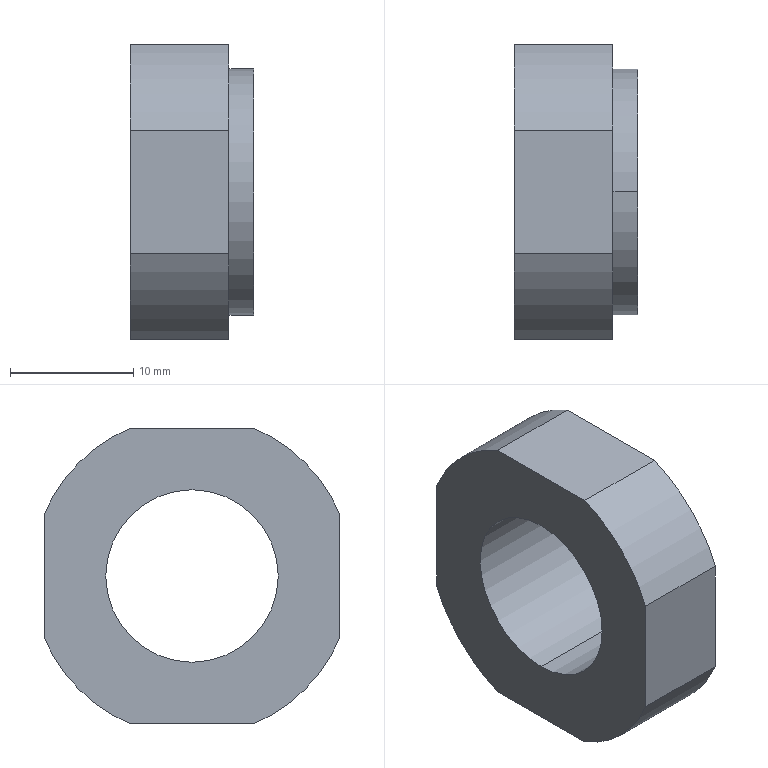Part | STEP file | PN_0054 locking nut | 1 solid | 15 faces | box 10 x 24 x 24 mm | volume 3121 mm3 | cylinder 8 | plane 7 | commonest cylinder face diameters 26 x4 14 x2 20 x2
STEP:
#1=CARTESIAN_POINT('',(0.,0.,0.));
#2=DIRECTION('',(0.,0.,1.));
#3=DIRECTION('',(1.,0.,0.));
#4=AXIS2_PLACEMENT_3D('',#1,#2,#3);
#5=CARTESIAN_POINT('',(-10.,0.,-7.));
#6=VERTEX_POINT('',#5);
#7=CARTESIAN_POINT('',(0.,0.,-7.));
#8=VERTEX_POINT('',#7);
#9=CARTESIAN_POINT('',(-10.,0.,-7.));
#10=DIRECTION('',(1.,0.,0.));
#11=VECTOR('',#10,1.);
#12=LINE('',#9,#11);
#13=CARTESIAN_POINT('',(-10.,0.,0.));
#14=DIRECTION('',(1.,0.,0.));
#15=DIRECTION('',(0.,0.,-1.));
#16=AXIS2_PLACEMENT_3D('',#13,#14,#15);
#17=CYLINDRICAL_SURFACE('',#16,7.);
#18=CARTESIAN_POINT('',(6.283,0.));
#19=DIRECTION('',(0.,1.));
#20=VECTOR('',#19,1.);
#21=LINE('',#18,#20);
#22=(GEOMETRIC_REPRESENTATION_CONTEXT(2)PARAMETRIC_REPRESENTATION_CONTEXT()REPRESENTATION_CONTEXT('',''));
#23=DEFINITIONAL_REPRESENTATION('',(#21),#22);
#24=PCURVE('',#17,#23);
#25=CARTESIAN_POINT('',(-10.,0.,0.));
#26=DIRECTION('',(1.,0.,0.));
#27=DIRECTION('',(0.,0.,-1.));
#28=AXIS2_PLACEMENT_3D('',#25,#26,#27);
#29=CYLINDRICAL_SURFACE('',#28,7.);
#30=CARTESIAN_POINT('',(0.,0.));
#31=DIRECTION('',(0.,1.));
#32=VECTOR('',#31,1.);
#33=LINE('',#30,#32);
#34=(GEOMETRIC_REPRESENTATION_CONTEXT(2)PARAMETRIC_REPRESENTATION_CONTEXT()REPRESENTATION_CONTEXT('',''));
#35=DEFINITIONAL_REPRESENTATION('',(#33),#34);
#36=PCURVE('',#29,#35);
#37=SURFACE_CURVE('',#12,(#24,#36),.PCURVE_S1.);
#38=EDGE_CURVE('',#6,#8,#37,.T.);
#39=ORIENTED_EDGE('',*,*,#38,.T.);
#40=CARTESIAN_POINT('',(0.,0.,7.));
#41=VERTEX_POINT('',#40);
#42=CARTESIAN_POINT('',(0.,0.,0.));
#43=DIRECTION('',(1.,0.,0.));
#44=DIRECTION('',(0.,0.,-1.));
#45=AXIS2_PLACEMENT_3D('',#42,#43,#44);
#46=CIRCLE('',#45,7.);
#47=CARTESIAN_POINT('',(0.,10.));
#48=DIRECTION('',(1.,0.));
#49=VECTOR('',#48,1.);
#50=LINE('',#47,#49);
#51=(GEOMETRIC_REPRESENTATION_CONTEXT(2)PARAMETRIC_REPRESENTATION_CONTEXT()REPRESENTATION_CONTEXT('',''));
#52=DEFINITIONAL_REPRESENTATION('',(#50),#51);
#53=PCURVE('',#17,#52);
#54=CARTESIAN_POINT('',(0.,0.,0.));
#55=DIRECTION('',(1.,0.,0.));
#56=DIRECTION('',(0.,0.,-1.));
#57=AXIS2_PLACEMENT_3D('',#54,#55,#56);
#58=PLANE('',#57);
#59=CARTESIAN_POINT('',(0.,0.));
#60=DIRECTION('',(1.,0.));
#61=AXIS2_PLACEMENT_2D('',#59,#60);
#62=CIRCLE('',#61,7.);
#63=(GEOMETRIC_REPRESENTATION_CONTEXT(2)PARAMETRIC_REPRESENTATION_CONTEXT()REPRESENTATION_CONTEXT('',''));
#64=DEFINITIONAL_REPRESENTATION('',(#62),#63);
#65=PCURVE('',#58,#64);
#66=SURFACE_CURVE('',#46,(#53,#65),.PCURVE_S1.);
#67=EDGE_CURVE('',#41,#8,#66,.T.);
#68=ORIENTED_EDGE('',*,*,#67,.F.);
#69=CARTESIAN_POINT('',(-10.,0.,7.));
#70=VERTEX_POINT('',#69);
#71=CARTESIAN_POINT('',(-10.,0.,7.));
#72=DIRECTION('',(1.,0.,0.));
#73=VECTOR('',#72,1.);
#74=LINE('',#71,#73);
#75=CARTESIAN_POINT('',(3.142,0.));
#76=DIRECTION('',(0.,1.));
#77=VECTOR('',#76,1.);
#78=LINE('',#75,#77);
#79=(GEOMETRIC_REPRESENTATION_CONTEXT(2)PARAMETRIC_REPRESENTATION_CONTEXT()REPRESENTATION_CONTEXT('',''));
#80=DEFINITIONAL_REPRESENTATION('',(#78),#79);
#81=PCURVE('',#17,#80);
#82=CARTESIAN_POINT('',(3.142,0.));
#83=DIRECTION('',(0.,1.));
#84=VECTOR('',#83,1.);
#85=LINE('',#82,#84);
#86=(GEOMETRIC_REPRESENTATION_CONTEXT(2)PARAMETRIC_REPRESENTATION_CONTEXT()REPRESENTATION_CONTEXT('',''));
#87=DEFINITIONAL_REPRESENTATION('',(#85),#86);
#88=PCURVE('',#29,#87);
#89=SURFACE_CURVE('',#74,(#81,#88),.PCURVE_S1.);
#90=EDGE_CURVE('',#70,#41,#89,.T.);
#91=ORIENTED_EDGE('',*,*,#90,.F.);
#92=CARTESIAN_POINT('',(-10.,0.,0.));
#93=DIRECTION('',(1.,0.,0.));
#94=DIRECTION('',(0.,0.,-1.));
#95=AXIS2_PLACEMENT_3D('',#92,#93,#94);
#96=CIRCLE('',#95,7.);
#97=CARTESIAN_POINT('',(0.,0.));
#98=DIRECTION('',(1.,0.));
#99=VECTOR('',#98,1.);
#100=LINE('',#97,#99);
#101=(GEOMETRIC_REPRESENTATION_CONTEXT(2)PARAMETRIC_REPRESENTATION_CONTEXT()REPRESENTATION_CONTEXT('',''));
#102=DEFINITIONAL_REPRESENTATION('',(#100),#101);
#103=PCURVE('',#17,#102);
#104=CARTESIAN_POINT('',(-10.,13.,0.));
#105=DIRECTION('',(-1.,0.,0.));
#106=DIRECTION('',(0.,0.,1.));
#107=AXIS2_PLACEMENT_3D('',#104,#105,#106);
#108=PLANE('',#107);
#109=CARTESIAN_POINT('',(-7.,-13.));
#110=CARTESIAN_POINT('',(-7.,-0.8756));
#111=CARTESIAN_POINT('',(3.5,-6.938));
#112=CARTESIAN_POINT('',(14.,-13.));
#113=CARTESIAN_POINT('',(3.5,-19.062));
#114=CARTESIAN_POINT('',(-7.,-25.124));
#115=CARTESIAN_POINT('',(-7.,-13.));
#116=(BOUNDED_CURVE()B_SPLINE_CURVE(2,(#109,#110,#111,#112,#113,#114,#115),.UNSPECIFIED.,.T.,.F.)B_SPLINE_CURVE_WITH_KNOTS((1,2,2,2,2,1),(-2.094,0.,2.094,4.189,6.283,8.378),.UNSPECIFIED.)CURVE()GEOMETRIC_REPRESENTATION_ITEM()RATIONAL_B_SPLINE_CURVE((1.,0.5,1.,0.5,1.,0.5,1.))REPRESENTATION_ITEM(''));
#117=(GEOMETRIC_REPRESENTATION_CONTEXT(2)PARAMETRIC_REPRESENTATION_CONTEXT()REPRESENTATION_CONTEXT('',''));
#118=DEFINITIONAL_REPRESENTATION('',(#116),#117);
#119=PCURVE('',#108,#118);
#120=SURFACE_CURVE('',#96,(#103,#119),.PCURVE_S1.);
#121=EDGE_CURVE('',#70,#6,#120,.T.);
#122=ORIENTED_EDGE('',*,*,#121,.T.);
#123=EDGE_LOOP('',(#39,#68,#91,#122));
#124=FACE_BOUND('',#123,.F.);
#125=ADVANCED_FACE('',(#124),#17,.F.);
#126=CARTESIAN_POINT('',(-2.,0.,-10.));
#127=VERTEX_POINT('',#126);
#128=CARTESIAN_POINT('',(-2.,0.,10.));
#129=VERTEX_POINT('',#128);
#130=CARTESIAN_POINT('',(-2.,0.,0.));
#131=DIRECTION('',(1.,0.,0.));
#132=DIRECTION('',(0.,0.,-1.));
#133=AXIS2_PLACEMENT_3D('',#130,#131,#132);
#134=CIRCLE('',#133,10.);
#135=CARTESIAN_POINT('',(0.,0.,0.));
#136=DIRECTION('',(1.,0.,0.));
#137=DIRECTION('',(0.,0.,-1.));
#138=AXIS2_PLACEMENT_3D('',#135,#136,#137);
#139=CYLINDRICAL_SURFACE('',#138,10.);
#140=CARTESIAN_POINT('',(0.,-2.));
#141=DIRECTION('',(1.,0.));
#142=VECTOR('',#141,1.);
#143=LINE('',#140,#142);
#144=(GEOMETRIC_REPRESENTATION_CONTEXT(2)PARAMETRIC_REPRESENTATION_CONTEXT()REPRESENTATION_CONTEXT('',''));
#145=DEFINITIONAL_REPRESENTATION('',(#143),#144);
#146=PCURVE('',#139,#145);
#147=CARTESIAN_POINT('',(-2.,10.,0.));
#148=DIRECTION('',(1.,0.,0.));
#149=DIRECTION('',(0.,0.,-1.));
#150=AXIS2_PLACEMENT_3D('',#147,#148,#149);
#151=PLANE('',#150);
#152=CARTESIAN_POINT('',(0.,-10.));
#153=DIRECTION('',(1.,0.));
#154=AXIS2_PLACEMENT_2D('',#152,#153);
#155=CIRCLE('',#154,10.);
#156=(GEOMETRIC_REPRESENTATION_CONTEXT(2)PARAMETRIC_REPRESENTATION_CONTEXT()REPRESENTATION_CONTEXT('',''));
#157=DEFINITIONAL_REPRESENTATION('',(#155),#156);
#158=PCURVE('',#151,#157);
#159=SURFACE_CURVE('',#134,(#146,#158),.PCURVE_S1.);
#160=EDGE_CURVE('',#127,#129,#159,.T.);
#161=ORIENTED_EDGE('',*,*,#160,.T.);
#162=CARTESIAN_POINT('',(0.,0.,10.));
#163=VERTEX_POINT('',#162);
#164=CARTESIAN_POINT('',(0.,0.,10.));
#165=DIRECTION('',(1.,0.,0.));
#166=VECTOR('',#165,1.);
#167=LINE('',#164,#166);
#168=CARTESIAN_POINT('',(3.142,0.));
#169=DIRECTION('',(0.,1.));
#170=VECTOR('',#169,1.);
#171=LINE('',#168,#170);
#172=(GEOMETRIC_REPRESENTATION_CONTEXT(2)PARAMETRIC_REPRESENTATION_CONTEXT()REPRESENTATION_CONTEXT('',''));
#173=DEFINITIONAL_REPRESENTATION('',(#171),#172);
#174=PCURVE('',#139,#173);
#175=CARTESIAN_POINT('',(0.,0.,0.));
#176=DIRECTION('',(1.,0.,0.));
#177=DIRECTION('',(0.,0.,-1.));
#178=AXIS2_PLACEMENT_3D('',#175,#176,#177);
#179=CYLINDRICAL_SURFACE('',#178,10.);
#180=CARTESIAN_POINT('',(3.142,0.));
#181=DIRECTION('',(0.,1.));
#182=VECTOR('',#181,1.);
#183=LINE('',#180,#182);
#184=(GEOMETRIC_REPRESENTATION_CONTEXT(2)PARAMETRIC_REPRESENTATION_CONTEXT()REPRESENTATION_CONTEXT('',''));
#185=DEFINITIONAL_REPRESENTATION('',(#183),#184);
#186=PCURVE('',#179,#185);
#187=SURFACE_CURVE('',#167,(#174,#186),.PCURVE_S1.);
#188=EDGE_CURVE('',#129,#163,#187,.T.);
#189=ORIENTED_EDGE('',*,*,#188,.T.);
#190=CARTESIAN_POINT('',(0.,0.,-10.));
#191=VERTEX_POINT('',#190);
#192=CARTESIAN_POINT('',(0.,0.,0.));
#193=DIRECTION('',(1.,0.,0.));
#194=DIRECTION('',(0.,0.,-1.));
#195=AXIS2_PLACEMENT_3D('',#192,#193,#194);
#196=CIRCLE('',#195,10.);
#197=CARTESIAN_POINT('',(0.,0.));
#198=DIRECTION('',(1.,0.));
#199=VECTOR('',#198,1.);
#200=LINE('',#197,#199);
#201=(GEOMETRIC_REPRESENTATION_CONTEXT(2)PARAMETRIC_REPRESENTATION_CONTEXT()REPRESENTATION_CONTEXT('',''));
#202=DEFINITIONAL_REPRESENTATION('',(#200),#201);
#203=PCURVE('',#139,#202);
#204=CARTESIAN_POINT('',(0.,0.));
#205=DIRECTION('',(1.,0.));
#206=AXIS2_PLACEMENT_2D('',#204,#205);
#207=CIRCLE('',#206,10.);
#208=(GEOMETRIC_REPRESENTATION_CONTEXT(2)PARAMETRIC_REPRESENTATION_CONTEXT()REPRESENTATION_CONTEXT('',''));
#209=DEFINITIONAL_REPRESENTATION('',(#207),#208);
#210=PCURVE('',#58,#209);
#211=SURFACE_CURVE('',#196,(#203,#210),.PCURVE_S1.);
#212=EDGE_CURVE('',#191,#163,#211,.T.);
#213=ORIENTED_EDGE('',*,*,#212,.F.);
#214=CARTESIAN_POINT('',(0.,0.,-10.));
#215=DIRECTION('',(1.,0.,0.));
#216=VECTOR('',#215,1.);
#217=LINE('',#214,#216);
#218=CARTESIAN_POINT('',(0.,0.));
#219=DIRECTION('',(0.,1.));
#220=VECTOR('',#219,1.);
#221=LINE('',#218,#220);
#222=(GEOMETRIC_REPRESENTATION_CONTEXT(2)PARAMETRIC_REPRESENTATION_CONTEXT()REPRESENTATION_CONTEXT('',''));
#223=DEFINITIONAL_REPRESENTATION('',(#221),#222);
#224=PCURVE('',#139,#223);
#225=CARTESIAN_POINT('',(6.283,0.));
#226=DIRECTION('',(0.,1.));
#227=VECTOR('',#226,1.);
#228=LINE('',#225,#227);
#229=(GEOMETRIC_REPRESENTATION_CONTEXT(2)PARAMETRIC_REPRESENTATION_CONTEXT()REPRESENTATION_CONTEXT('',''));
#230=DEFINITIONAL_REPRESENTATION('',(#228),#229);
#231=PCURVE('',#179,#230);
#232=SURFACE_CURVE('',#217,(#224,#231),.PCURVE_S1.);
#233=EDGE_CURVE('',#127,#191,#232,.T.);
#234=ORIENTED_EDGE('',*,*,#233,.F.);
#235=EDGE_LOOP('',(#161,#189,#213,#234));
#236=FACE_BOUND('',#235,.T.);
#237=ADVANCED_FACE('',(#236),#139,.T.);
#238=CARTESIAN_POINT('',(-2.,5.,12.));
#239=VERTEX_POINT('',#238);
#240=CARTESIAN_POINT('',(-10.,5.,12.));
#241=VERTEX_POINT('',#240);
#242=CARTESIAN_POINT('',(0.,5.,12.));
#243=DIRECTION('',(-1.,0.,0.));
#244=VECTOR('',#243,1.);
#245=LINE('',#242,#244);
#246=CARTESIAN_POINT('',(0.,0.,0.));
#247=DIRECTION('',(1.,0.,0.));
#248=DIRECTION('',(0.,0.,-1.));
#249=AXIS2_PLACEMENT_3D('',#246,#247,#248);
#250=CYLINDRICAL_SURFACE('',#249,13.);
#251=CARTESIAN_POINT('',(2.747,0.));
#252=DIRECTION('',(0.,-1.));
#253=VECTOR('',#252,1.);
#254=LINE('',#251,#253);
#255=(GEOMETRIC_REPRESENTATION_CONTEXT(2)PARAMETRIC_REPRESENTATION_CONTEXT()REPRESENTATION_CONTEXT('',''));
#256=DEFINITIONAL_REPRESENTATION('',(#254),#255);
#257=PCURVE('',#250,#256);
#258=CARTESIAN_POINT('',(0.,17.205,12.));
#259=DIRECTION('',(0.,0.,-1.));
#260=DIRECTION('',(0.,1.,0.));
#261=AXIS2_PLACEMENT_3D('',#258,#259,#260);
#262=PLANE('',#261);
#263=CARTESIAN_POINT('',(-12.205,0.));
#264=DIRECTION('',(0.,-1.));
#265=VECTOR('',#264,1.);
#266=LINE('',#263,#265);
#267=(GEOMETRIC_REPRESENTATION_CONTEXT(2)PARAMETRIC_REPRESENTATION_CONTEXT()REPRESENTATION_CONTEXT('',''));
#268=DEFINITIONAL_REPRESENTATION('',(#266),#267);
#269=PCURVE('',#262,#268);
#270=SURFACE_CURVE('',#245,(#257,#269),.PCURVE_S1.);
#271=EDGE_CURVE('',#239,#241,#270,.T.);
#272=ORIENTED_EDGE('',*,*,#271,.F.);
#273=CARTESIAN_POINT('',(-2.,12.,5.));
#274=VERTEX_POINT('',#273);
#275=CARTESIAN_POINT('',(-2.,0.,0.));
#276=DIRECTION('',(1.,0.,0.));
#277=DIRECTION('',(0.,0.,-1.));
#278=AXIS2_PLACEMENT_3D('',#275,#276,#277);
#279=CIRCLE('',#278,13.);
#280=CARTESIAN_POINT('',(0.,-2.));
#281=DIRECTION('',(1.,0.));
#282=VECTOR('',#281,1.);
#283=LINE('',#280,#282);
#284=(GEOMETRIC_REPRESENTATION_CONTEXT(2)PARAMETRIC_REPRESENTATION_CONTEXT()REPRESENTATION_CONTEXT('',''));
#285=DEFINITIONAL_REPRESENTATION('',(#283),#284);
#286=PCURVE('',#250,#285);
#287=CARTESIAN_POINT('',(0.,-10.));
#288=DIRECTION('',(1.,0.));
#289=AXIS2_PLACEMENT_2D('',#287,#288);
#290=CIRCLE('',#289,13.);
#291=(GEOMETRIC_REPRESENTATION_CONTEXT(2)PARAMETRIC_REPRESENTATION_CONTEXT()REPRESENTATION_CONTEXT('',''));
#292=DEFINITIONAL_REPRESENTATION('',(#290),#291);
#293=PCURVE('',#151,#292);
#294=SURFACE_CURVE('',#279,(#286,#293),.PCURVE_S1.);
#295=EDGE_CURVE('',#274,#239,#294,.T.);
#296=ORIENTED_EDGE('',*,*,#295,.F.);
#297=CARTESIAN_POINT('',(-10.,12.,5.));
#298=VERTEX_POINT('',#297);
#299=CARTESIAN_POINT('',(0.,12.,5.));
#300=DIRECTION('',(1.,0.,0.));
#301=VECTOR('',#300,1.);
#302=LINE('',#299,#301);
#303=CARTESIAN_POINT('',(1.966,0.));
#304=DIRECTION('',(0.,1.));
#305=VECTOR('',#304,1.);
#306=LINE('',#303,#305);
#307=(GEOMETRIC_REPRESENTATION_CONTEXT(2)PARAMETRIC_REPRESENTATION_CONTEXT()REPRESENTATION_CONTEXT('',''));
#308=DEFINITIONAL_REPRESENTATION('',(#306),#307);
#309=PCURVE('',#250,#308);
#310=CARTESIAN_POINT('',(0.,12.,-20.296));
#311=DIRECTION('',(0.,-1.,0.));
#312=DIRECTION('',(0.,0.,-1.));
#313=AXIS2_PLACEMENT_3D('',#310,#311,#312);
#314=PLANE('',#313);
#315=CARTESIAN_POINT('',(-25.296,0.));
#316=DIRECTION('',(0.,1.));
#317=VECTOR('',#316,1.);
#318=LINE('',#315,#317);
#319=(GEOMETRIC_REPRESENTATION_CONTEXT(2)PARAMETRIC_REPRESENTATION_CONTEXT()REPRESENTATION_CONTEXT('',''));
#320=DEFINITIONAL_REPRESENTATION('',(#318),#319);
#321=PCURVE('',#314,#320);
#322=SURFACE_CURVE('',#302,(#309,#321),.PCURVE_S1.);
#323=EDGE_CURVE('',#298,#274,#322,.T.);
#324=ORIENTED_EDGE('',*,*,#323,.F.);
#325=CARTESIAN_POINT('',(-10.,0.,0.));
#326=DIRECTION('',(1.,0.,0.));
#327=DIRECTION('',(0.,0.,-1.));
#328=AXIS2_PLACEMENT_3D('',#325,#326,#327);
#329=CIRCLE('',#328,13.);
#330=CARTESIAN_POINT('',(0.,-10.));
#331=DIRECTION('',(1.,0.));
#332=VECTOR('',#331,1.);
#333=LINE('',#330,#332);
#334=(GEOMETRIC_REPRESENTATION_CONTEXT(2)PARAMETRIC_REPRESENTATION_CONTEXT()REPRESENTATION_CONTEXT('',''));
#335=DEFINITIONAL_REPRESENTATION('',(#333),#334);
#336=PCURVE('',#250,#335);
#337=CARTESIAN_POINT('',(-13.,-13.));
#338=CARTESIAN_POINT('',(-13.,9.517));
#339=CARTESIAN_POINT('',(6.5,-1.742));
#340=CARTESIAN_POINT('',(26.,-13.));
#341=CARTESIAN_POINT('',(6.5,-24.258));
#342=CARTESIAN_POINT('',(-13.,-35.517));
#343=CARTESIAN_POINT('',(-13.,-13.));
#344=(BOUNDED_CURVE()B_SPLINE_CURVE(2,(#337,#338,#339,#340,#341,#342,#343),.UNSPECIFIED.,.T.,.F.)B_SPLINE_CURVE_WITH_KNOTS((1,2,2,2,2,1),(-2.094,0.,2.094,4.189,6.283,8.378),.UNSPECIFIED.)CURVE()GEOMETRIC_REPRESENTATION_ITEM()RATIONAL_B_SPLINE_CURVE((1.,0.5,1.,0.5,1.,0.5,1.))REPRESENTATION_ITEM(''));
#345=(GEOMETRIC_REPRESENTATION_CONTEXT(2)PARAMETRIC_REPRESENTATION_CONTEXT()REPRESENTATION_CONTEXT('',''));
#346=DEFINITIONAL_REPRESENTATION('',(#344),#345);
#347=PCURVE('',#108,#346);
#348=SURFACE_CURVE('',#329,(#336,#347),.PCURVE_S1.);
#349=EDGE_CURVE('',#298,#241,#348,.T.);
#350=ORIENTED_EDGE('',*,*,#349,.T.);
#351=EDGE_LOOP('',(#272,#296,#324,#350));
#352=FACE_BOUND('',#351,.T.);
#353=ADVANCED_FACE('',(#352),#250,.T.);
#354=CARTESIAN_POINT('',(-2.,-5.,-12.));
#355=VERTEX_POINT('',#354);
#356=CARTESIAN_POINT('',(-10.,-5.,-12.));
#357=VERTEX_POINT('',#356);
#358=CARTESIAN_POINT('',(0.,-5.,-12.));
#359=DIRECTION('',(-1.,0.,0.));
#360=VECTOR('',#359,1.);
#361=LINE('',#358,#360);
#362=CARTESIAN_POINT('',(0.,0.,0.));
#363=DIRECTION('',(1.,0.,0.));
#364=DIRECTION('',(0.,0.,-1.));
#365=AXIS2_PLACEMENT_3D('',#362,#363,#364);
#366=CYLINDRICAL_SURFACE('',#365,13.);
#367=CARTESIAN_POINT('',(5.888,0.));
#368=DIRECTION('',(0.,-1.));
#369=VECTOR('',#368,1.);
#370=LINE('',#367,#369);
#371=(GEOMETRIC_REPRESENTATION_CONTEXT(2)PARAMETRIC_REPRESENTATION_CONTEXT()REPRESENTATION_CONTEXT('',''));
#372=DEFINITIONAL_REPRESENTATION('',(#370),#371);
#373=PCURVE('',#366,#372);
#374=CARTESIAN_POINT('',(0.,17.205,-12.));
#375=DIRECTION('',(0.,0.,1.));
#376=DIRECTION('',(0.,-1.,0.));
#377=AXIS2_PLACEMENT_3D('',#374,#375,#376);
#378=PLANE('',#377);
#379=CARTESIAN_POINT('',(22.205,0.));
#380=DIRECTION('',(0.,-1.));
#381=VECTOR('',#380,1.);
#382=LINE('',#379,#381);
#383=(GEOMETRIC_REPRESENTATION_CONTEXT(2)PARAMETRIC_REPRESENTATION_CONTEXT()REPRESENTATION_CONTEXT('',''));
#384=DEFINITIONAL_REPRESENTATION('',(#382),#383);
#385=PCURVE('',#378,#384);
#386=SURFACE_CURVE('',#361,(#373,#385),.PCURVE_S1.);
#387=EDGE_CURVE('',#355,#357,#386,.T.);
#388=ORIENTED_EDGE('',*,*,#387,.F.);
#389=CARTESIAN_POINT('',(-2.,-12.,-5.));
#390=VERTEX_POINT('',#389);
#391=CARTESIAN_POINT('',(-2.,0.,0.));
#392=DIRECTION('',(1.,0.,0.));
#393=DIRECTION('',(0.,0.,-1.));
#394=AXIS2_PLACEMENT_3D('',#391,#392,#393);
#395=CIRCLE('',#394,13.);
#396=CARTESIAN_POINT('',(0.,-2.));
#397=DIRECTION('',(1.,0.));
#398=VECTOR('',#397,1.);
#399=LINE('',#396,#398);
#400=(GEOMETRIC_REPRESENTATION_CONTEXT(2)PARAMETRIC_REPRESENTATION_CONTEXT()REPRESENTATION_CONTEXT('',''));
#401=DEFINITIONAL_REPRESENTATION('',(#399),#400);
#402=PCURVE('',#366,#401);
#403=CARTESIAN_POINT('',(0.,-10.));
#404=DIRECTION('',(1.,0.));
#405=AXIS2_PLACEMENT_2D('',#403,#404);
#406=CIRCLE('',#405,13.);
#407=(GEOMETRIC_REPRESENTATION_CONTEXT(2)PARAMETRIC_REPRESENTATION_CONTEXT()REPRESENTATION_CONTEXT('',''));
#408=DEFINITIONAL_REPRESENTATION('',(#406),#407);
#409=PCURVE('',#151,#408);
#410=SURFACE_CURVE('',#395,(#402,#409),.PCURVE_S1.);
#411=EDGE_CURVE('',#390,#355,#410,.T.);
#412=ORIENTED_EDGE('',*,*,#411,.F.);
#413=CARTESIAN_POINT('',(-10.,-12.,-5.));
#414=VERTEX_POINT('',#413);
#415=CARTESIAN_POINT('',(0.,-12.,-5.));
#416=DIRECTION('',(1.,0.,0.));
#417=VECTOR('',#416,1.);
#418=LINE('',#415,#417);
#419=CARTESIAN_POINT('',(5.107,0.));
#420=DIRECTION('',(0.,1.));
#421=VECTOR('',#420,1.);
#422=LINE('',#419,#421);
#423=(GEOMETRIC_REPRESENTATION_CONTEXT(2)PARAMETRIC_REPRESENTATION_CONTEXT()REPRESENTATION_CONTEXT('',''));
#424=DEFINITIONAL_REPRESENTATION('',(#422),#423);
#425=PCURVE('',#366,#424);
#426=CARTESIAN_POINT('',(0.,-12.,-20.296));
#427=DIRECTION('',(0.,1.,0.));
#428=DIRECTION('',(0.,0.,1.));
#429=AXIS2_PLACEMENT_3D('',#426,#427,#428);
#430=PLANE('',#429);
#431=CARTESIAN_POINT('',(15.296,0.));
#432=DIRECTION('',(0.,1.));
#433=VECTOR('',#432,1.);
#434=LINE('',#431,#433);
#435=(GEOMETRIC_REPRESENTATION_CONTEXT(2)PARAMETRIC_REPRESENTATION_CONTEXT()REPRESENTATION_CONTEXT('',''));
#436=DEFINITIONAL_REPRESENTATION('',(#434),#435);
#437=PCURVE('',#430,#436);
#438=SURFACE_CURVE('',#418,(#425,#437),.PCURVE_S1.);
#439=EDGE_CURVE('',#414,#390,#438,.T.);
#440=ORIENTED_EDGE('',*,*,#439,.F.);
#441=CARTESIAN_POINT('',(-10.,0.,0.));
#442=DIRECTION('',(1.,0.,0.));
#443=DIRECTION('',(0.,0.,-1.));
#444=AXIS2_PLACEMENT_3D('',#441,#442,#443);
#445=CIRCLE('',#444,13.);
#446=CARTESIAN_POINT('',(0.,-10.));
#447=DIRECTION('',(1.,0.));
#448=VECTOR('',#447,1.);
#449=LINE('',#446,#448);
#450=(GEOMETRIC_REPRESENTATION_CONTEXT(2)PARAMETRIC_REPRESENTATION_CONTEXT()REPRESENTATION_CONTEXT('',''));
#451=DEFINITIONAL_REPRESENTATION('',(#449),#450);
#452=PCURVE('',#366,#451);
#453=CARTESIAN_POINT('',(-13.,-13.));
#454=CARTESIAN_POINT('',(-13.,9.517));
#455=CARTESIAN_POINT('',(6.5,-1.742));
#456=CARTESIAN_POINT('',(26.,-13.));
#457=CARTESIAN_POINT('',(6.5,-24.258));
#458=CARTESIAN_POINT('',(-13.,-35.517));
#459=CARTESIAN_POINT('',(-13.,-13.));
#460=(BOUNDED_CURVE()B_SPLINE_CURVE(2,(#453,#454,#455,#456,#457,#458,#459),.UNSPECIFIED.,.T.,.F.)B_SPLINE_CURVE_WITH_KNOTS((1,2,2,2,2,1),(-2.094,0.,2.094,4.189,6.283,8.378),.UNSPECIFIED.)CURVE()GEOMETRIC_REPRESENTATION_ITEM()RATIONAL_B_SPLINE_CURVE((1.,0.5,1.,0.5,1.,0.5,1.))REPRESENTATION_ITEM(''));
#461=(GEOMETRIC_REPRESENTATION_CONTEXT(2)PARAMETRIC_REPRESENTATION_CONTEXT()REPRESENTATION_CONTEXT('',''));
#462=DEFINITIONAL_REPRESENTATION('',(#460),#461);
#463=PCURVE('',#108,#462);
#464=SURFACE_CURVE('',#445,(#452,#463),.PCURVE_S1.);
#465=EDGE_CURVE('',#414,#357,#464,.T.);
#466=ORIENTED_EDGE('',*,*,#465,.T.);
#467=EDGE_LOOP('',(#388,#412,#440,#466));
#468=FACE_BOUND('',#467,.T.);
#469=ADVANCED_FACE('',(#468),#366,.T.);
#470=CARTESIAN_POINT('',(-10.,-5.,12.));
#471=VERTEX_POINT('',#470);
#472=CARTESIAN_POINT('',(-2.,-5.,12.));
#473=VERTEX_POINT('',#472);
#474=CARTESIAN_POINT('',(0.,-5.,12.));
#475=DIRECTION('',(1.,0.,0.));
#476=VECTOR('',#475,1.);
#477=LINE('',#474,#476);
#478=CARTESIAN_POINT('',(0.,0.,0.));
#479=DIRECTION('',(1.,0.,0.));
#480=DIRECTION('',(0.,0.,-1.));
#481=AXIS2_PLACEMENT_3D('',#478,#479,#480);
#482=CYLINDRICAL_SURFACE('',#481,13.);
#483=CARTESIAN_POINT('',(3.536,0.));
#484=DIRECTION('',(0.,1.));
#485=VECTOR('',#484,1.);
#486=LINE('',#483,#485);
#487=(GEOMETRIC_REPRESENTATION_CONTEXT(2)PARAMETRIC_REPRESENTATION_CONTEXT()REPRESENTATION_CONTEXT('',''));
#488=DEFINITIONAL_REPRESENTATION('',(#486),#487);
#489=PCURVE('',#482,#488);
#490=CARTESIAN_POINT('',(-22.205,0.));
#491=DIRECTION('',(0.,1.));
#492=VECTOR('',#491,1.);
#493=LINE('',#490,#492);
#494=(GEOMETRIC_REPRESENTATION_CONTEXT(2)PARAMETRIC_REPRESENTATION_CONTEXT()REPRESENTATION_CONTEXT('',''));
#495=DEFINITIONAL_REPRESENTATION('',(#493),#494);
#496=PCURVE('',#262,#495);
#497=SURFACE_CURVE('',#477,(#489,#496),.PCURVE_S1.);
#498=EDGE_CURVE('',#471,#473,#497,.T.);
#499=ORIENTED_EDGE('',*,*,#498,.F.);
#500=CARTESIAN_POINT('',(-10.,-12.,5.));
#501=VERTEX_POINT('',#500);
#502=CARTESIAN_POINT('',(-10.,0.,0.));
#503=DIRECTION('',(1.,0.,0.));
#504=DIRECTION('',(0.,0.,-1.));
#505=AXIS2_PLACEMENT_3D('',#502,#503,#504);
#506=CIRCLE('',#505,13.);
#507=CARTESIAN_POINT('',(0.,-10.));
#508=DIRECTION('',(1.,0.));
#509=VECTOR('',#508,1.);
#510=LINE('',#507,#509);
#511=(GEOMETRIC_REPRESENTATION_CONTEXT(2)PARAMETRIC_REPRESENTATION_CONTEXT()REPRESENTATION_CONTEXT('',''));
#512=DEFINITIONAL_REPRESENTATION('',(#510),#511);
#513=PCURVE('',#482,#512);
#514=CARTESIAN_POINT('',(-13.,-13.));
#515=CARTESIAN_POINT('',(-13.,9.517));
#516=CARTESIAN_POINT('',(6.5,-1.742));
#517=CARTESIAN_POINT('',(26.,-13.));
#518=CARTESIAN_POINT('',(6.5,-24.258));
#519=CARTESIAN_POINT('',(-13.,-35.517));
#520=CARTESIAN_POINT('',(-13.,-13.));
#521=(BOUNDED_CURVE()B_SPLINE_CURVE(2,(#514,#515,#516,#517,#518,#519,#520),.UNSPECIFIED.,.T.,.F.)B_SPLINE_CURVE_WITH_KNOTS((1,2,2,2,2,1),(-2.094,0.,2.094,4.189,6.283,8.378),.UNSPECIFIED.)CURVE()GEOMETRIC_REPRESENTATION_ITEM()RATIONAL_B_SPLINE_CURVE((1.,0.5,1.,0.5,1.,0.5,1.))REPRESENTATION_ITEM(''));
#522=(GEOMETRIC_REPRESENTATION_CONTEXT(2)PARAMETRIC_REPRESENTATION_CONTEXT()REPRESENTATION_CONTEXT('',''));
#523=DEFINITIONAL_REPRESENTATION('',(#521),#522);
#524=PCURVE('',#108,#523);
#525=SURFACE_CURVE('',#506,(#513,#524),.PCURVE_S1.);
#526=EDGE_CURVE('',#471,#501,#525,.T.);
#527=ORIENTED_EDGE('',*,*,#526,.T.);
#528=CARTESIAN_POINT('',(-2.,-12.,5.));
#529=VERTEX_POINT('',#528);
#530=CARTESIAN_POINT('',(0.,-12.,5.));
#531=DIRECTION('',(-1.,0.,0.));
#532=VECTOR('',#531,1.);
#533=LINE('',#530,#532);
#534=CARTESIAN_POINT('',(4.318,0.));
#535=DIRECTION('',(0.,-1.));
#536=VECTOR('',#535,1.);
#537=LINE('',#534,#536);
#538=(GEOMETRIC_REPRESENTATION_CONTEXT(2)PARAMETRIC_REPRESENTATION_CONTEXT()REPRESENTATION_CONTEXT('',''));
#539=DEFINITIONAL_REPRESENTATION('',(#537),#538);
#540=PCURVE('',#482,#539);
#541=CARTESIAN_POINT('',(25.296,0.));
#542=DIRECTION('',(0.,-1.));
#543=VECTOR('',#542,1.);
#544=LINE('',#541,#543);
#545=(GEOMETRIC_REPRESENTATION_CONTEXT(2)PARAMETRIC_REPRESENTATION_CONTEXT()REPRESENTATION_CONTEXT('',''));
#546=DEFINITIONAL_REPRESENTATION('',(#544),#545);
#547=PCURVE('',#430,#546);
#548=SURFACE_CURVE('',#533,(#540,#547),.PCURVE_S1.);
#549=EDGE_CURVE('',#529,#501,#548,.T.);
#550=ORIENTED_EDGE('',*,*,#549,.F.);
#551=CARTESIAN_POINT('',(-2.,0.,0.));
#552=DIRECTION('',(1.,0.,0.));
#553=DIRECTION('',(0.,0.,-1.));
#554=AXIS2_PLACEMENT_3D('',#551,#552,#553);
#555=CIRCLE('',#554,13.);
#556=CARTESIAN_POINT('',(0.,-2.));
#557=DIRECTION('',(1.,0.));
#558=VECTOR('',#557,1.);
#559=LINE('',#556,#558);
#560=(GEOMETRIC_REPRESENTATION_CONTEXT(2)PARAMETRIC_REPRESENTATION_CONTEXT()REPRESENTATION_CONTEXT('',''));
#561=DEFINITIONAL_REPRESENTATION('',(#559),#560);
#562=PCURVE('',#482,#561);
#563=CARTESIAN_POINT('',(0.,-10.));
#564=DIRECTION('',(1.,0.));
#565=AXIS2_PLACEMENT_2D('',#563,#564);
#566=CIRCLE('',#565,13.);
#567=(GEOMETRIC_REPRESENTATION_CONTEXT(2)PARAMETRIC_REPRESENTATION_CONTEXT()REPRESENTATION_CONTEXT('',''));
#568=DEFINITIONAL_REPRESENTATION('',(#566),#567);
#569=PCURVE('',#151,#568);
#570=SURFACE_CURVE('',#555,(#562,#569),.PCURVE_S1.);
#571=EDGE_CURVE('',#473,#529,#570,.T.);
#572=ORIENTED_EDGE('',*,*,#571,.F.);
#573=EDGE_LOOP('',(#499,#527,#550,#572));
#574=FACE_BOUND('',#573,.T.);
#575=ADVANCED_FACE('',(#574),#482,.T.);
#576=CARTESIAN_POINT('',(0.,0.,0.));
#577=DIRECTION('',(1.,0.,0.));
#578=DIRECTION('',(0.,0.,-1.));
#579=AXIS2_PLACEMENT_3D('',#576,#577,#578);
#580=CIRCLE('',#579,7.);
#581=CARTESIAN_POINT('',(0.,0.));
#582=DIRECTION('',(1.,0.));
#583=AXIS2_PLACEMENT_2D('',#581,#582);
#584=CIRCLE('',#583,7.);
#585=(GEOMETRIC_REPRESENTATION_CONTEXT(2)PARAMETRIC_REPRESENTATION_CONTEXT()REPRESENTATION_CONTEXT('',''));
#586=DEFINITIONAL_REPRESENTATION('',(#584),#585);
#587=PCURVE('',#58,#586);
#588=CARTESIAN_POINT('',(0.,10.));
#589=DIRECTION('',(1.,0.));
#590=VECTOR('',#589,1.);
#591=LINE('',#588,#590);
#592=(GEOMETRIC_REPRESENTATION_CONTEXT(2)PARAMETRIC_REPRESENTATION_CONTEXT()REPRESENTATION_CONTEXT('',''));
#593=DEFINITIONAL_REPRESENTATION('',(#591),#592);
#594=PCURVE('',#29,#593);
#595=SURFACE_CURVE('',#580,(#587,#594),.PCURVE_S1.);
#596=EDGE_CURVE('',#8,#41,#595,.T.);
#597=ORIENTED_EDGE('',*,*,#596,.F.);
#598=ORIENTED_EDGE('',*,*,#67,.F.);
#599=EDGE_LOOP('',(#597,#598));
#600=FACE_BOUND('',#599,.T.);
#601=ORIENTED_EDGE('',*,*,#212,.T.);
#602=CARTESIAN_POINT('',(0.,0.,0.));
#603=DIRECTION('',(1.,0.,0.));
#604=DIRECTION('',(0.,0.,-1.));
#605=AXIS2_PLACEMENT_3D('',#602,#603,#604);
#606=CIRCLE('',#605,10.);
#607=CARTESIAN_POINT('',(0.,0.));
#608=DIRECTION('',(1.,0.));
#609=AXIS2_PLACEMENT_2D('',#607,#608);
#610=CIRCLE('',#609,10.);
#611=(GEOMETRIC_REPRESENTATION_CONTEXT(2)PARAMETRIC_REPRESENTATION_CONTEXT()REPRESENTATION_CONTEXT('',''));
#612=DEFINITIONAL_REPRESENTATION('',(#610),#611);
#613=PCURVE('',#58,#612);
#614=CARTESIAN_POINT('',(0.,0.));
#615=DIRECTION('',(1.,0.));
#616=VECTOR('',#615,1.);
#617=LINE('',#614,#616);
#618=(GEOMETRIC_REPRESENTATION_CONTEXT(2)PARAMETRIC_REPRESENTATION_CONTEXT()REPRESENTATION_CONTEXT('',''));
#619=DEFINITIONAL_REPRESENTATION('',(#617),#618);
#620=PCURVE('',#179,#619);
#621=SURFACE_CURVE('',#606,(#613,#620),.PCURVE_S1.);
#622=EDGE_CURVE('',#163,#191,#621,.T.);
#623=ORIENTED_EDGE('',*,*,#622,.T.);
#624=EDGE_LOOP('',(#601,#623));
#625=FACE_BOUND('',#624,.T.);
#626=ADVANCED_FACE('',(#600,#625),#58,.T.);
#627=ORIENTED_EDGE('',*,*,#188,.F.);
#628=CARTESIAN_POINT('',(-2.,0.,0.));
#629=DIRECTION('',(1.,0.,0.));
#630=DIRECTION('',(0.,0.,-1.));
#631=AXIS2_PLACEMENT_3D('',#628,#629,#630);
#632=CIRCLE('',#631,10.);
#633=CARTESIAN_POINT('',(0.,-2.));
#634=DIRECTION('',(1.,0.));
#635=VECTOR('',#634,1.);
#636=LINE('',#633,#635);
#637=(GEOMETRIC_REPRESENTATION_CONTEXT(2)PARAMETRIC_REPRESENTATION_CONTEXT()REPRESENTATION_CONTEXT('',''));
#638=DEFINITIONAL_REPRESENTATION('',(#636),#637);
#639=PCURVE('',#179,#638);
#640=CARTESIAN_POINT('',(0.,-10.));
#641=DIRECTION('',(1.,0.));
#642=AXIS2_PLACEMENT_2D('',#640,#641);
#643=CIRCLE('',#642,10.);
#644=(GEOMETRIC_REPRESENTATION_CONTEXT(2)PARAMETRIC_REPRESENTATION_CONTEXT()REPRESENTATION_CONTEXT('',''));
#645=DEFINITIONAL_REPRESENTATION('',(#643),#644);
#646=PCURVE('',#151,#645);
#647=SURFACE_CURVE('',#632,(#639,#646),.PCURVE_S1.);
#648=EDGE_CURVE('',#129,#127,#647,.T.);
#649=ORIENTED_EDGE('',*,*,#648,.T.);
#650=ORIENTED_EDGE('',*,*,#233,.T.);
#651=ORIENTED_EDGE('',*,*,#622,.F.);
#652=EDGE_LOOP('',(#627,#649,#650,#651));
#653=FACE_BOUND('',#652,.T.);
#654=ADVANCED_FACE('',(#653),#179,.T.);
#655=CARTESIAN_POINT('',(-2.,10.,12.));
#656=DIRECTION('',(0.,1.,0.));
#657=VECTOR('',#656,1.);
#658=LINE('',#655,#657);
#659=CARTESIAN_POINT('',(-12.,0.));
#660=DIRECTION('',(0.,1.));
#661=VECTOR('',#660,1.);
#662=LINE('',#659,#661);
#663=(GEOMETRIC_REPRESENTATION_CONTEXT(2)PARAMETRIC_REPRESENTATION_CONTEXT()REPRESENTATION_CONTEXT('',''));
#664=DEFINITIONAL_REPRESENTATION('',(#662),#663);
#665=PCURVE('',#151,#664);
#666=CARTESIAN_POINT('',(-7.205,-2.));
#667=DIRECTION('',(1.,0.));
#668=VECTOR('',#667,1.);
#669=LINE('',#666,#668);
#670=(GEOMETRIC_REPRESENTATION_CONTEXT(2)PARAMETRIC_REPRESENTATION_CONTEXT()REPRESENTATION_CONTEXT('',''));
#671=DEFINITIONAL_REPRESENTATION('',(#669),#670);
#672=PCURVE('',#262,#671);
#673=SURFACE_CURVE('',#658,(#665,#672),.PCURVE_S1.);
#674=EDGE_CURVE('',#473,#239,#673,.T.);
#675=ORIENTED_EDGE('',*,*,#674,.F.);
#676=ORIENTED_EDGE('',*,*,#571,.T.);
#677=CARTESIAN_POINT('',(-2.,-12.,0.));
#678=DIRECTION('',(0.,0.,1.));
#679=VECTOR('',#678,1.);
#680=LINE('',#677,#679);
#681=CARTESIAN_POINT('',(0.,-22.));
#682=DIRECTION('',(-1.,0.));
#683=VECTOR('',#682,1.);
#684=LINE('',#681,#683);
#685=(GEOMETRIC_REPRESENTATION_CONTEXT(2)PARAMETRIC_REPRESENTATION_CONTEXT()REPRESENTATION_CONTEXT('',''));
#686=DEFINITIONAL_REPRESENTATION('',(#684),#685);
#687=PCURVE('',#151,#686);
#688=CARTESIAN_POINT('',(20.296,-2.));
#689=DIRECTION('',(1.,0.));
#690=VECTOR('',#689,1.);
#691=LINE('',#688,#690);
#692=(GEOMETRIC_REPRESENTATION_CONTEXT(2)PARAMETRIC_REPRESENTATION_CONTEXT()REPRESENTATION_CONTEXT('',''));
#693=DEFINITIONAL_REPRESENTATION('',(#691),#692);
#694=PCURVE('',#430,#693);
#695=SURFACE_CURVE('',#680,(#687,#694),.PCURVE_S1.);
#696=EDGE_CURVE('',#390,#529,#695,.T.);
#697=ORIENTED_EDGE('',*,*,#696,.F.);
#698=ORIENTED_EDGE('',*,*,#411,.T.);
#699=CARTESIAN_POINT('',(-2.,5.,-12.));
#700=VERTEX_POINT('',#699);
#701=CARTESIAN_POINT('',(-2.,10.,-12.));
#702=DIRECTION('',(0.,-1.,0.));
#703=VECTOR('',#702,1.);
#704=LINE('',#701,#703);
#705=CARTESIAN_POINT('',(12.,0.));
#706=DIRECTION('',(0.,-1.));
#707=VECTOR('',#706,1.);
#708=LINE('',#705,#707);
#709=(GEOMETRIC_REPRESENTATION_CONTEXT(2)PARAMETRIC_REPRESENTATION_CONTEXT()REPRESENTATION_CONTEXT('',''));
#710=DEFINITIONAL_REPRESENTATION('',(#708),#709);
#711=PCURVE('',#151,#710);
#712=CARTESIAN_POINT('',(7.205,-2.));
#713=DIRECTION('',(1.,0.));
#714=VECTOR('',#713,1.);
#715=LINE('',#712,#714);
#716=(GEOMETRIC_REPRESENTATION_CONTEXT(2)PARAMETRIC_REPRESENTATION_CONTEXT()REPRESENTATION_CONTEXT('',''));
#717=DEFINITIONAL_REPRESENTATION('',(#715),#716);
#718=PCURVE('',#378,#717);
#719=SURFACE_CURVE('',#704,(#711,#718),.PCURVE_S1.);
#720=EDGE_CURVE('',#700,#355,#719,.T.);
#721=ORIENTED_EDGE('',*,*,#720,.F.);
#722=CARTESIAN_POINT('',(-2.,12.,-5.));
#723=VERTEX_POINT('',#722);
#724=CARTESIAN_POINT('',(-2.,0.,0.));
#725=DIRECTION('',(1.,0.,0.));
#726=DIRECTION('',(0.,0.,-1.));
#727=AXIS2_PLACEMENT_3D('',#724,#725,#726);
#728=CIRCLE('',#727,13.);
#729=CARTESIAN_POINT('',(0.,-10.));
#730=DIRECTION('',(1.,0.));
#731=AXIS2_PLACEMENT_2D('',#729,#730);
#732=CIRCLE('',#731,13.);
#733=(GEOMETRIC_REPRESENTATION_CONTEXT(2)PARAMETRIC_REPRESENTATION_CONTEXT()REPRESENTATION_CONTEXT('',''));
#734=DEFINITIONAL_REPRESENTATION('',(#732),#733);
#735=PCURVE('',#151,#734);
#736=CARTESIAN_POINT('',(0.,0.,0.));
#737=DIRECTION('',(1.,0.,0.));
#738=DIRECTION('',(0.,0.,-1.));
#739=AXIS2_PLACEMENT_3D('',#736,#737,#738);
#740=CYLINDRICAL_SURFACE('',#739,13.);
#741=CARTESIAN_POINT('',(0.,-2.));
#742=DIRECTION('',(1.,0.));
#743=VECTOR('',#742,1.);
#744=LINE('',#741,#743);
#745=(GEOMETRIC_REPRESENTATION_CONTEXT(2)PARAMETRIC_REPRESENTATION_CONTEXT()REPRESENTATION_CONTEXT('',''));
#746=DEFINITIONAL_REPRESENTATION('',(#744),#745);
#747=PCURVE('',#740,#746);
#748=SURFACE_CURVE('',#728,(#735,#747),.PCURVE_S1.);
#749=EDGE_CURVE('',#700,#723,#748,.T.);
#750=ORIENTED_EDGE('',*,*,#749,.T.);
#751=CARTESIAN_POINT('',(-2.,12.,0.));
#752=DIRECTION('',(0.,0.,-1.));
#753=VECTOR('',#752,1.);
#754=LINE('',#751,#753);
#755=CARTESIAN_POINT('',(0.,2.));
#756=DIRECTION('',(1.,0.));
#757=VECTOR('',#756,1.);
#758=LINE('',#755,#757);
#759=(GEOMETRIC_REPRESENTATION_CONTEXT(2)PARAMETRIC_REPRESENTATION_CONTEXT()REPRESENTATION_CONTEXT('',''));
#760=DEFINITIONAL_REPRESENTATION('',(#758),#759);
#761=PCURVE('',#151,#760);
#762=CARTESIAN_POINT('',(-20.296,-2.));
#763=DIRECTION('',(1.,0.));
#764=VECTOR('',#763,1.);
#765=LINE('',#762,#764);
#766=(GEOMETRIC_REPRESENTATION_CONTEXT(2)PARAMETRIC_REPRESENTATION_CONTEXT()REPRESENTATION_CONTEXT('',''));
#767=DEFINITIONAL_REPRESENTATION('',(#765),#766);
#768=PCURVE('',#314,#767);
#769=SURFACE_CURVE('',#754,(#761,#768),.PCURVE_S1.);
#770=EDGE_CURVE('',#274,#723,#769,.T.);
#771=ORIENTED_EDGE('',*,*,#770,.F.);
#772=ORIENTED_EDGE('',*,*,#295,.T.);
#773=EDGE_LOOP('',(#675,#676,#697,#698,#721,#750,#771,#772));
#774=FACE_BOUND('',#773,.T.);
#775=ORIENTED_EDGE('',*,*,#160,.F.);
#776=ORIENTED_EDGE('',*,*,#648,.F.);
#777=EDGE_LOOP('',(#775,#776));
#778=FACE_BOUND('',#777,.T.);
#779=ADVANCED_FACE('',(#774,#778),#151,.T.);
#780=CARTESIAN_POINT('',(-10.,5.,-12.));
#781=VERTEX_POINT('',#780);
#782=CARTESIAN_POINT('',(0.,5.,-12.));
#783=DIRECTION('',(1.,0.,0.));
#784=VECTOR('',#783,1.);
#785=LINE('',#782,#784);
#786=CARTESIAN_POINT('',(0.3948,0.));
#787=DIRECTION('',(0.,1.));
#788=VECTOR('',#787,1.);
#789=LINE('',#786,#788);
#790=(GEOMETRIC_REPRESENTATION_CONTEXT(2)PARAMETRIC_REPRESENTATION_CONTEXT()REPRESENTATION_CONTEXT('',''));
#791=DEFINITIONAL_REPRESENTATION('',(#789),#790);
#792=PCURVE('',#740,#791);
#793=CARTESIAN_POINT('',(12.205,0.));
#794=DIRECTION('',(0.,1.));
#795=VECTOR('',#794,1.);
#796=LINE('',#793,#795);
#797=(GEOMETRIC_REPRESENTATION_CONTEXT(2)PARAMETRIC_REPRESENTATION_CONTEXT()REPRESENTATION_CONTEXT('',''));
#798=DEFINITIONAL_REPRESENTATION('',(#796),#797);
#799=PCURVE('',#378,#798);
#800=SURFACE_CURVE('',#785,(#792,#799),.PCURVE_S1.);
#801=EDGE_CURVE('',#781,#700,#800,.T.);
#802=ORIENTED_EDGE('',*,*,#801,.F.);
#803=CARTESIAN_POINT('',(-10.,12.,-5.));
#804=VERTEX_POINT('',#803);
#805=CARTESIAN_POINT('',(-10.,0.,0.));
#806=DIRECTION('',(1.,0.,0.));
#807=DIRECTION('',(0.,0.,-1.));
#808=AXIS2_PLACEMENT_3D('',#805,#806,#807);
#809=CIRCLE('',#808,13.);
#810=CARTESIAN_POINT('',(0.,-10.));
#811=DIRECTION('',(1.,0.));
#812=VECTOR('',#811,1.);
#813=LINE('',#810,#812);
#814=(GEOMETRIC_REPRESENTATION_CONTEXT(2)PARAMETRIC_REPRESENTATION_CONTEXT()REPRESENTATION_CONTEXT('',''));
#815=DEFINITIONAL_REPRESENTATION('',(#813),#814);
#816=PCURVE('',#740,#815);
#817=CARTESIAN_POINT('',(-13.,-13.));
#818=CARTESIAN_POINT('',(-13.,9.517));
#819=CARTESIAN_POINT('',(6.5,-1.742));
#820=CARTESIAN_POINT('',(26.,-13.));
#821=CARTESIAN_POINT('',(6.5,-24.258));
#822=CARTESIAN_POINT('',(-13.,-35.517));
#823=CARTESIAN_POINT('',(-13.,-13.));
#824=(BOUNDED_CURVE()B_SPLINE_CURVE(2,(#817,#818,#819,#820,#821,#822,#823),.UNSPECIFIED.,.T.,.F.)B_SPLINE_CURVE_WITH_KNOTS((1,2,2,2,2,1),(-2.094,0.,2.094,4.189,6.283,8.378),.UNSPECIFIED.)CURVE()GEOMETRIC_REPRESENTATION_ITEM()RATIONAL_B_SPLINE_CURVE((1.,0.5,1.,0.5,1.,0.5,1.))REPRESENTATION_ITEM(''));
#825=(GEOMETRIC_REPRESENTATION_CONTEXT(2)PARAMETRIC_REPRESENTATION_CONTEXT()REPRESENTATION_CONTEXT('',''));
#826=DEFINITIONAL_REPRESENTATION('',(#824),#825);
#827=PCURVE('',#108,#826);
#828=SURFACE_CURVE('',#809,(#816,#827),.PCURVE_S1.);
#829=EDGE_CURVE('',#781,#804,#828,.T.);
#830=ORIENTED_EDGE('',*,*,#829,.T.);
#831=CARTESIAN_POINT('',(0.,12.,-5.));
#832=DIRECTION('',(-1.,0.,0.));
#833=VECTOR('',#832,1.);
#834=LINE('',#831,#833);
#835=CARTESIAN_POINT('',(1.176,0.));
#836=DIRECTION('',(0.,-1.));
#837=VECTOR('',#836,1.);
#838=LINE('',#835,#837);
#839=(GEOMETRIC_REPRESENTATION_CONTEXT(2)PARAMETRIC_REPRESENTATION_CONTEXT()REPRESENTATION_CONTEXT('',''));
#840=DEFINITIONAL_REPRESENTATION('',(#838),#839);
#841=PCURVE('',#740,#840);
#842=CARTESIAN_POINT('',(-15.296,0.));
#843=DIRECTION('',(0.,-1.));
#844=VECTOR('',#843,1.);
#845=LINE('',#842,#844);
#846=(GEOMETRIC_REPRESENTATION_CONTEXT(2)PARAMETRIC_REPRESENTATION_CONTEXT()REPRESENTATION_CONTEXT('',''));
#847=DEFINITIONAL_REPRESENTATION('',(#845),#846);
#848=PCURVE('',#314,#847);
#849=SURFACE_CURVE('',#834,(#841,#848),.PCURVE_S1.);
#850=EDGE_CURVE('',#723,#804,#849,.T.);
#851=ORIENTED_EDGE('',*,*,#850,.F.);
#852=ORIENTED_EDGE('',*,*,#749,.F.);
#853=EDGE_LOOP('',(#802,#830,#851,#852));
#854=FACE_BOUND('',#853,.T.);
#855=ADVANCED_FACE('',(#854),#740,.T.);
#856=CARTESIAN_POINT('',(-10.,13.,12.));
#857=DIRECTION('',(0.,-1.,0.));
#858=VECTOR('',#857,1.);
#859=LINE('',#856,#858);
#860=CARTESIAN_POINT('',(12.,0.));
#861=DIRECTION('',(0.,-1.));
#862=VECTOR('',#861,1.);
#863=LINE('',#860,#862);
#864=(GEOMETRIC_REPRESENTATION_CONTEXT(2)PARAMETRIC_REPRESENTATION_CONTEXT()REPRESENTATION_CONTEXT('',''));
#865=DEFINITIONAL_REPRESENTATION('',(#863),#864);
#866=PCURVE('',#108,#865);
#867=CARTESIAN_POINT('',(-4.205,-10.));
#868=DIRECTION('',(-1.,0.));
#869=VECTOR('',#868,1.);
#870=LINE('',#867,#869);
#871=(GEOMETRIC_REPRESENTATION_CONTEXT(2)PARAMETRIC_REPRESENTATION_CONTEXT()REPRESENTATION_CONTEXT('',''));
#872=DEFINITIONAL_REPRESENTATION('',(#870),#871);
#873=PCURVE('',#262,#872);
#874=SURFACE_CURVE('',#859,(#866,#873),.PCURVE_S1.);
#875=EDGE_CURVE('',#241,#471,#874,.T.);
#876=ORIENTED_EDGE('',*,*,#875,.F.);
#877=ORIENTED_EDGE('',*,*,#349,.F.);
#878=CARTESIAN_POINT('',(-10.,12.,0.));
#879=DIRECTION('',(0.,0.,1.));
#880=VECTOR('',#879,1.);
#881=LINE('',#878,#880);
#882=CARTESIAN_POINT('',(0.,-1.));
#883=DIRECTION('',(1.,0.));
#884=VECTOR('',#883,1.);
#885=LINE('',#882,#884);
#886=(GEOMETRIC_REPRESENTATION_CONTEXT(2)PARAMETRIC_REPRESENTATION_CONTEXT()REPRESENTATION_CONTEXT('',''));
#887=DEFINITIONAL_REPRESENTATION('',(#885),#886);
#888=PCURVE('',#108,#887);
#889=CARTESIAN_POINT('',(-20.296,-10.));
#890=DIRECTION('',(-1.,0.));
#891=VECTOR('',#890,1.);
#892=LINE('',#889,#891);
#893=(GEOMETRIC_REPRESENTATION_CONTEXT(2)PARAMETRIC_REPRESENTATION_CONTEXT()REPRESENTATION_CONTEXT('',''));
#894=DEFINITIONAL_REPRESENTATION('',(#892),#893);
#895=PCURVE('',#314,#894);
#896=SURFACE_CURVE('',#881,(#888,#895),.PCURVE_S1.);
#897=EDGE_CURVE('',#804,#298,#896,.T.);
#898=ORIENTED_EDGE('',*,*,#897,.F.);
#899=ORIENTED_EDGE('',*,*,#829,.F.);
#900=CARTESIAN_POINT('',(-10.,13.,-12.));
#901=DIRECTION('',(0.,1.,0.));
#902=VECTOR('',#901,1.);
#903=LINE('',#900,#902);
#904=CARTESIAN_POINT('',(-12.,0.));
#905=DIRECTION('',(0.,1.));
#906=VECTOR('',#905,1.);
#907=LINE('',#904,#906);
#908=(GEOMETRIC_REPRESENTATION_CONTEXT(2)PARAMETRIC_REPRESENTATION_CONTEXT()REPRESENTATION_CONTEXT('',''));
#909=DEFINITIONAL_REPRESENTATION('',(#907),#908);
#910=PCURVE('',#108,#909);
#911=CARTESIAN_POINT('',(4.205,-10.));
#912=DIRECTION('',(-1.,0.));
#913=VECTOR('',#912,1.);
#914=LINE('',#911,#913);
#915=(GEOMETRIC_REPRESENTATION_CONTEXT(2)PARAMETRIC_REPRESENTATION_CONTEXT()REPRESENTATION_CONTEXT('',''));
#916=DEFINITIONAL_REPRESENTATION('',(#914),#915);
#917=PCURVE('',#378,#916);
#918=SURFACE_CURVE('',#903,(#910,#917),.PCURVE_S1.);
#919=EDGE_CURVE('',#357,#781,#918,.T.);
#920=ORIENTED_EDGE('',*,*,#919,.F.);
#921=ORIENTED_EDGE('',*,*,#465,.F.);
#922=CARTESIAN_POINT('',(-10.,-12.,0.));
#923=DIRECTION('',(0.,0.,-1.));
#924=VECTOR('',#923,1.);
#925=LINE('',#922,#924);
#926=CARTESIAN_POINT('',(0.,-25.));
#927=DIRECTION('',(-1.,0.));
#928=VECTOR('',#927,1.);
#929=LINE('',#926,#928);
#930=(GEOMETRIC_REPRESENTATION_CONTEXT(2)PARAMETRIC_REPRESENTATION_CONTEXT()REPRESENTATION_CONTEXT('',''));
#931=DEFINITIONAL_REPRESENTATION('',(#929),#930);
#932=PCURVE('',#108,#931);
#933=CARTESIAN_POINT('',(20.296,-10.));
#934=DIRECTION('',(-1.,0.));
#935=VECTOR('',#934,1.);
#936=LINE('',#933,#935);
#937=(GEOMETRIC_REPRESENTATION_CONTEXT(2)PARAMETRIC_REPRESENTATION_CONTEXT()REPRESENTATION_CONTEXT('',''));
#938=DEFINITIONAL_REPRESENTATION('',(#936),#937);
#939=PCURVE('',#430,#938);
#940=SURFACE_CURVE('',#925,(#932,#939),.PCURVE_S1.);
#941=EDGE_CURVE('',#501,#414,#940,.T.);
#942=ORIENTED_EDGE('',*,*,#941,.F.);
#943=ORIENTED_EDGE('',*,*,#526,.F.);
#944=EDGE_LOOP('',(#876,#877,#898,#899,#920,#921,#942,#943));
#945=FACE_BOUND('',#944,.T.);
#946=CARTESIAN_POINT('',(-10.,0.,0.));
#947=DIRECTION('',(1.,0.,0.));
#948=DIRECTION('',(0.,0.,-1.));
#949=AXIS2_PLACEMENT_3D('',#946,#947,#948);
#950=CIRCLE('',#949,7.);
#951=CARTESIAN_POINT('',(-7.,-13.));
#952=CARTESIAN_POINT('',(-7.,-0.8756));
#953=CARTESIAN_POINT('',(3.5,-6.938));
#954=CARTESIAN_POINT('',(14.,-13.));
#955=CARTESIAN_POINT('',(3.5,-19.062));
#956=CARTESIAN_POINT('',(-7.,-25.124));
#957=CARTESIAN_POINT('',(-7.,-13.));
#958=(BOUNDED_CURVE()B_SPLINE_CURVE(2,(#951,#952,#953,#954,#955,#956,#957),.UNSPECIFIED.,.T.,.F.)B_SPLINE_CURVE_WITH_KNOTS((1,2,2,2,2,1),(-2.094,0.,2.094,4.189,6.283,8.378),.UNSPECIFIED.)CURVE()GEOMETRIC_REPRESENTATION_ITEM()RATIONAL_B_SPLINE_CURVE((1.,0.5,1.,0.5,1.,0.5,1.))REPRESENTATION_ITEM(''));
#959=(GEOMETRIC_REPRESENTATION_CONTEXT(2)PARAMETRIC_REPRESENTATION_CONTEXT()REPRESENTATION_CONTEXT('',''));
#960=DEFINITIONAL_REPRESENTATION('',(#958),#959);
#961=PCURVE('',#108,#960);
#962=CARTESIAN_POINT('',(0.,0.));
#963=DIRECTION('',(1.,0.));
#964=VECTOR('',#963,1.);
#965=LINE('',#962,#964);
#966=(GEOMETRIC_REPRESENTATION_CONTEXT(2)PARAMETRIC_REPRESENTATION_CONTEXT()REPRESENTATION_CONTEXT('',''));
#967=DEFINITIONAL_REPRESENTATION('',(#965),#966);
#968=PCURVE('',#29,#967);
#969=SURFACE_CURVE('',#950,(#961,#968),.PCURVE_S1.);
#970=EDGE_CURVE('',#6,#70,#969,.T.);
#971=ORIENTED_EDGE('',*,*,#970,.T.);
#972=ORIENTED_EDGE('',*,*,#121,.T.);
#973=EDGE_LOOP('',(#971,#972));
#974=FACE_BOUND('',#973,.T.);
#975=ADVANCED_FACE('',(#945,#974),#108,.T.);
#976=ORIENTED_EDGE('',*,*,#596,.F.);
#977=ORIENTED_EDGE('',*,*,#38,.F.);
#978=ORIENTED_EDGE('',*,*,#970,.T.);
#979=ORIENTED_EDGE('',*,*,#90,.T.);
#980=EDGE_LOOP('',(#976,#977,#978,#979));
#981=FACE_BOUND('',#980,.F.);
#982=ADVANCED_FACE('',(#981),#29,.F.);
#983=ORIENTED_EDGE('',*,*,#850,.T.);
#984=ORIENTED_EDGE('',*,*,#897,.T.);
#985=ORIENTED_EDGE('',*,*,#323,.T.);
#986=ORIENTED_EDGE('',*,*,#770,.T.);
#987=EDGE_LOOP('',(#983,#984,#985,#986));
#988=FACE_BOUND('',#987,.T.);
#989=ADVANCED_FACE('',(#988),#314,.F.);
#990=ORIENTED_EDGE('',*,*,#549,.T.);
#991=ORIENTED_EDGE('',*,*,#941,.T.);
#992=ORIENTED_EDGE('',*,*,#439,.T.);
#993=ORIENTED_EDGE('',*,*,#696,.T.);
#994=EDGE_LOOP('',(#990,#991,#992,#993));
#995=FACE_BOUND('',#994,.T.);
#996=ADVANCED_FACE('',(#995),#430,.F.);
#997=ORIENTED_EDGE('',*,*,#387,.T.);
#998=ORIENTED_EDGE('',*,*,#919,.T.);
#999=ORIENTED_EDGE('',*,*,#801,.T.);
#1000=ORIENTED_EDGE('',*,*,#720,.T.);
#1001=EDGE_LOOP('',(#997,#998,#999,#1000));
#1002=FACE_BOUND('',#1001,.T.);
#1003=ADVANCED_FACE('',(#1002),#378,.F.);
#1004=ORIENTED_EDGE('',*,*,#271,.T.);
#1005=ORIENTED_EDGE('',*,*,#875,.T.);
#1006=ORIENTED_EDGE('',*,*,#498,.T.);
#1007=ORIENTED_EDGE('',*,*,#674,.T.);
#1008=EDGE_LOOP('',(#1004,#1005,#1006,#1007));
#1009=FACE_BOUND('',#1008,.T.);
#1010=ADVANCED_FACE('',(#1009),#262,.F.);
#1011=CLOSED_SHELL('',(#125,#237,#353,#469,#575,#626,#654,#779,#855,#975,#982,#989,#996,#1003,#1010));
#1012=MANIFOLD_SOLID_BREP('',#1011);
#1013=(LENGTH_UNIT()NAMED_UNIT(*)SI_UNIT(.MILLI.,.METRE.));
#1014=UNCERTAINTY_MEASURE_WITH_UNIT(LENGTH_MEASURE(0.0000001),#1013,'','');
#1015=(NAMED_UNIT(*)PLANE_ANGLE_UNIT()SI_UNIT($,.RADIAN.));
#1016=(NAMED_UNIT(*)SI_UNIT($,.STERADIAN.)SOLID_ANGLE_UNIT());
#1017=(GEOMETRIC_REPRESENTATION_CONTEXT(3)GLOBAL_UNCERTAINTY_ASSIGNED_CONTEXT((#1014))GLOBAL_UNIT_ASSIGNED_CONTEXT((#1013,#1015,#1016))REPRESENTATION_CONTEXT('',''));
#1018=ADVANCED_BREP_SHAPE_REPRESENTATION('',(#4,#1012),#1017);